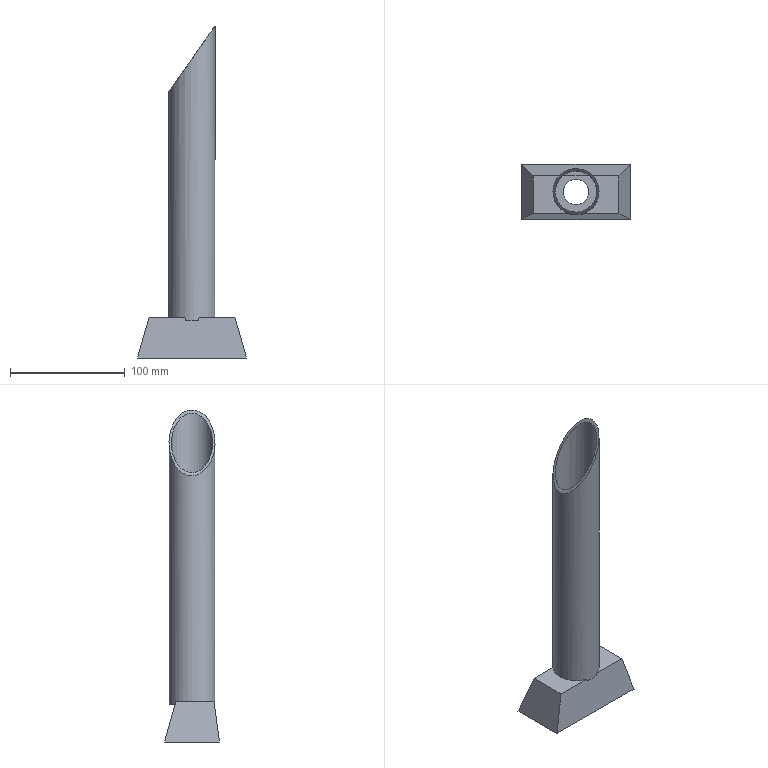Part | NX | features EXTRUDE 4, DATUM_CSYS 3, SKETCH 3, EXTRACT_DATUM_PLANE 2, SHELL 2, DRAFT 1, UNITE 1 | 1 solid | 19 faces | box 95 x 48 x 289.397 mm | volume 75187 mm3 | plane 12 | spline 4 | cylinder 3 | commonest cylinder face diameters 22.182 x1 36.182 x1 40.182 x1
STEP:
#1=CARTESIAN_POINT('',(5.362,-19.362,33.));
#2=VERTEX_POINT('',#1);
#3=CARTESIAN_POINT('',(6.29,-19.081,35.));
#4=VERTEX_POINT('',#3);
#5=CARTESIAN_POINT('',(0.,0.,170.769));
#6=DIRECTION('',(0.,0.9903,-0.1392));
#7=DIRECTION('',(0.,-0.1392,-0.9903));
#8=AXIS2_PLACEMENT_3D('',#5,#6,#7);
#9=ELLIPSE('',#8,144.36,20.091);
#10=EDGE_CURVE('',#2,#4,#9,.F.);
#11=ORIENTED_EDGE('',*,*,#10,.F.);
#12=CARTESIAN_POINT('',(-5.362,-19.362,33.));
#13=VERTEX_POINT('',#12);
#14=CARTESIAN_POINT('',(0.000000047,-19.362,33.));
#15=DIRECTION('',(1.,0.,0.));
#16=VECTOR('',#15,1000.);
#17=LINE('',#14,#16);
#18=EDGE_CURVE('',#13,#2,#17,.T.);
#19=ORIENTED_EDGE('',*,*,#18,.F.);
#20=CARTESIAN_POINT('',(-6.29,-19.081,35.));
#21=VERTEX_POINT('',#20);
#22=CARTESIAN_POINT('',(0.,0.,170.769));
#23=DIRECTION('',(0.,0.9903,-0.1392));
#24=DIRECTION('',(0.,-0.1392,-0.9903));
#25=AXIS2_PLACEMENT_3D('',#22,#23,#24);
#26=ELLIPSE('',#25,144.36,20.091);
#27=EDGE_CURVE('',#21,#13,#26,.F.);
#28=ORIENTED_EDGE('',*,*,#27,.F.);
#29=CARTESIAN_POINT('',(-37.464,-19.081,35.));
#30=VERTEX_POINT('',#29);
#31=CARTESIAN_POINT('',(0.000000047,-19.081,35.));
#32=DIRECTION('',(1.,0.,0.));
#33=VECTOR('',#32,1000.);
#34=LINE('',#31,#33);
#35=EDGE_CURVE('',#30,#21,#34,.T.);
#36=ORIENTED_EDGE('',*,*,#35,.F.);
#37=CARTESIAN_POINT('',(-47.5,-24.,0.));
#38=VERTEX_POINT('',#37);
#39=CARTESIAN_POINT('',(-37.464,-19.081,35.));
#40=CARTESIAN_POINT('',(-40.809,-20.721,23.333));
#41=CARTESIAN_POINT('',(-44.155,-22.36,11.667));
#42=CARTESIAN_POINT('',(-47.5,-24.,0.));
#43=B_SPLINE_CURVE_WITH_KNOTS('',3,(#39,#40,#41,#42),.UNSPECIFIED.,.F.,.F.,(4,4),(0.,0.03674),.UNSPECIFIED.);
#44=EDGE_CURVE('',#30,#38,#43,.T.);
#45=ORIENTED_EDGE('',*,*,#44,.T.);
#46=CARTESIAN_POINT('',(47.5,-24.,0.));
#47=VERTEX_POINT('',#46);
#48=CARTESIAN_POINT('',(0.000000047,-24.,0.));
#49=DIRECTION('',(1.,0.,0.));
#50=VECTOR('',#49,1000.);
#51=LINE('',#48,#50);
#52=EDGE_CURVE('',#38,#47,#51,.T.);
#53=ORIENTED_EDGE('',*,*,#52,.T.);
#54=CARTESIAN_POINT('',(37.463,-19.081,35.));
#55=VERTEX_POINT('',#54);
#56=CARTESIAN_POINT('',(37.463,-19.081,35.));
#57=CARTESIAN_POINT('',(40.809,-20.721,23.333));
#58=CARTESIAN_POINT('',(44.154,-22.36,11.667));
#59=CARTESIAN_POINT('',(47.5,-24.,0.));
#60=B_SPLINE_CURVE_WITH_KNOTS('',3,(#56,#57,#58,#59),.UNSPECIFIED.,.F.,.F.,(4,4),(0.,0.03674),.UNSPECIFIED.);
#61=EDGE_CURVE('',#55,#47,#60,.T.);
#62=ORIENTED_EDGE('',*,*,#61,.F.);
#63=CARTESIAN_POINT('',(0.000000047,-19.081,35.));
#64=DIRECTION('',(1.,0.,0.));
#65=VECTOR('',#64,1000.);
#66=LINE('',#63,#65);
#67=EDGE_CURVE('',#4,#55,#66,.T.);
#68=ORIENTED_EDGE('',*,*,#67,.F.);
#69=EDGE_LOOP('',(#11,#19,#28,#36,#45,#53,#62,#68));
#70=FACE_BOUND('',#69,.T.);
#71=CARTESIAN_POINT('',(0.000000047,-24.,0.));
#72=DIRECTION('',(0.,0.9903,-0.1392));
#73=DIRECTION('',(0.,0.1392,0.9903));
#74=AXIS2_PLACEMENT_3D('',#71,#72,#73);
#75=PLANE('',#74);
#76=ADVANCED_FACE('',(#70),#75,.F.);
#77=ORIENTED_EDGE('',*,*,#35,.T.);
#78=CARTESIAN_POINT('',(-14.445,13.964,35.));
#79=VERTEX_POINT('',#78);
#80=CARTESIAN_POINT('',(0.,0.,35.));
#81=DIRECTION('',(0.,0.,1.));
#82=DIRECTION('',(1.,0.,0.));
#83=AXIS2_PLACEMENT_3D('',#80,#81,#82);
#84=CIRCLE('',#83,20.091);
#85=EDGE_CURVE('',#21,#79,#84,.F.);
#86=ORIENTED_EDGE('',*,*,#85,.T.);
#87=CARTESIAN_POINT('',(-37.463,13.964,35.));
#88=VERTEX_POINT('',#87);
#89=CARTESIAN_POINT('',(0.000000047,13.964,35.));
#90=DIRECTION('',(-1.,0.,0.));
#91=VECTOR('',#90,1000.);
#92=LINE('',#89,#91);
#93=EDGE_CURVE('',#79,#88,#92,.T.);
#94=ORIENTED_EDGE('',*,*,#93,.T.);
#95=CARTESIAN_POINT('',(-37.463,13.964,35.));
#96=CARTESIAN_POINT('',(-37.463,2.949,35.));
#97=CARTESIAN_POINT('',(-37.463,-8.066,35.));
#98=CARTESIAN_POINT('',(-37.464,-19.081,35.));
#99=B_SPLINE_CURVE_WITH_KNOTS('',3,(#95,#96,#97,#98),.UNSPECIFIED.,.F.,.F.,(4,4),(0.,0.03304),.UNSPECIFIED.);
#100=EDGE_CURVE('',#88,#30,#99,.T.);
#101=ORIENTED_EDGE('',*,*,#100,.T.);
#102=EDGE_LOOP('',(#77,#86,#94,#101));
#103=FACE_BOUND('',#102,.T.);
#104=CARTESIAN_POINT('',(-47.5,-0.000000093,35.));
#105=DIRECTION('',(0.,0.,1.));
#106=DIRECTION('',(1.,0.,0.));
#107=AXIS2_PLACEMENT_3D('',#104,#105,#106);
#108=PLANE('',#107);
#109=ADVANCED_FACE('',(#103),#108,.T.);
#110=CARTESIAN_POINT('',(11.091,0.,35.));
#111=VERTEX_POINT('',#110);
#112=CARTESIAN_POINT('',(0.,0.,35.));
#113=DIRECTION('',(0.,0.,1.));
#114=DIRECTION('',(1.,0.,0.));
#115=AXIS2_PLACEMENT_3D('',#112,#113,#114);
#116=CIRCLE('',#115,11.091);
#117=EDGE_CURVE('',#111,#111,#116,.F.);
#118=ORIENTED_EDGE('',*,*,#117,.T.);
#119=EDGE_LOOP('',(#118));
#120=FACE_BOUND('',#119,.T.);
#121=CARTESIAN_POINT('',(11.502,13.964,35.));
#122=VERTEX_POINT('',#121);
#123=CARTESIAN_POINT('',(-11.502,13.964,35.));
#124=VERTEX_POINT('',#123);
#125=CARTESIAN_POINT('',(0.,0.,35.));
#126=DIRECTION('',(0.,0.,1.));
#127=DIRECTION('',(1.,0.,0.));
#128=AXIS2_PLACEMENT_3D('',#125,#126,#127);
#129=CIRCLE('',#128,18.091);
#130=EDGE_CURVE('',#122,#124,#129,.F.);
#131=ORIENTED_EDGE('',*,*,#130,.F.);
#132=CARTESIAN_POINT('',(0.000000047,13.964,35.));
#133=DIRECTION('',(-1.,0.,0.));
#134=VECTOR('',#133,1000.);
#135=LINE('',#132,#134);
#136=EDGE_CURVE('',#122,#124,#135,.T.);
#137=ORIENTED_EDGE('',*,*,#136,.T.);
#138=EDGE_LOOP('',(#131,#137));
#139=FACE_BOUND('',#138,.T.);
#140=CARTESIAN_POINT('',(-47.5,-0.000000093,35.));
#141=DIRECTION('',(0.,0.,1.));
#142=DIRECTION('',(1.,0.,0.));
#143=AXIS2_PLACEMENT_3D('',#140,#141,#142);
#144=PLANE('',#143);
#145=ADVANCED_FACE('',(#120,#139),#144,.T.);
#146=CARTESIAN_POINT('',(-13.868,14.537,33.));
#147=VERTEX_POINT('',#146);
#148=CARTESIAN_POINT('',(0.,0.,83.698));
#149=DIRECTION('',(0.,-0.9613,-0.2756));
#150=DIRECTION('',(0.,0.2756,-0.9613));
#151=AXIS2_PLACEMENT_3D('',#148,#149,#150);
#152=ELLIPSE('',#151,72.889,20.091);
#153=EDGE_CURVE('',#147,#79,#152,.F.);
#154=ORIENTED_EDGE('',*,*,#153,.F.);
#155=CARTESIAN_POINT('',(-10.768,14.537,33.));
#156=VERTEX_POINT('',#155);
#157=CARTESIAN_POINT('',(0.000000047,14.537,33.));
#158=DIRECTION('',(-1.,0.,0.));
#159=VECTOR('',#158,1000.);
#160=LINE('',#157,#159);
#161=EDGE_CURVE('',#156,#147,#160,.T.);
#162=ORIENTED_EDGE('',*,*,#161,.F.);
#163=CARTESIAN_POINT('',(0.,0.,83.698));
#164=DIRECTION('',(0.,-0.9613,-0.2756));
#165=DIRECTION('',(0.,0.2756,-0.9613));
#166=AXIS2_PLACEMENT_3D('',#163,#164,#165);
#167=ELLIPSE('',#166,65.633,18.091);
#168=EDGE_CURVE('',#124,#156,#167,.T.);
#169=ORIENTED_EDGE('',*,*,#168,.F.);
#170=ORIENTED_EDGE('',*,*,#136,.F.);
#171=CARTESIAN_POINT('',(10.768,14.537,33.));
#172=VERTEX_POINT('',#171);
#173=CARTESIAN_POINT('',(0.,0.,83.698));
#174=DIRECTION('',(0.,-0.9613,-0.2756));
#175=DIRECTION('',(0.,0.2756,-0.9613));
#176=AXIS2_PLACEMENT_3D('',#173,#174,#175);
#177=ELLIPSE('',#176,65.633,18.091);
#178=EDGE_CURVE('',#172,#122,#177,.T.);
#179=ORIENTED_EDGE('',*,*,#178,.F.);
#180=CARTESIAN_POINT('',(13.868,14.537,33.));
#181=VERTEX_POINT('',#180);
#182=CARTESIAN_POINT('',(0.000000047,14.537,33.));
#183=DIRECTION('',(-1.,0.,0.));
#184=VECTOR('',#183,1000.);
#185=LINE('',#182,#184);
#186=EDGE_CURVE('',#181,#172,#185,.T.);
#187=ORIENTED_EDGE('',*,*,#186,.F.);
#188=CARTESIAN_POINT('',(14.445,13.964,35.));
#189=VERTEX_POINT('',#188);
#190=CARTESIAN_POINT('',(0.,0.,83.698));
#191=DIRECTION('',(0.,-0.9613,-0.2756));
#192=DIRECTION('',(0.,0.2756,-0.9613));
#193=AXIS2_PLACEMENT_3D('',#190,#191,#192);
#194=ELLIPSE('',#193,72.889,20.091);
#195=EDGE_CURVE('',#189,#181,#194,.F.);
#196=ORIENTED_EDGE('',*,*,#195,.F.);
#197=CARTESIAN_POINT('',(37.463,13.964,35.));
#198=VERTEX_POINT('',#197);
#199=CARTESIAN_POINT('',(0.000000047,13.964,35.));
#200=DIRECTION('',(-1.,0.,0.));
#201=VECTOR('',#200,1000.);
#202=LINE('',#199,#201);
#203=EDGE_CURVE('',#198,#189,#202,.T.);
#204=ORIENTED_EDGE('',*,*,#203,.F.);
#205=CARTESIAN_POINT('',(47.5,24.,0.));
#206=VERTEX_POINT('',#205);
#207=CARTESIAN_POINT('',(37.463,13.964,35.));
#208=CARTESIAN_POINT('',(40.809,17.309,23.333));
#209=CARTESIAN_POINT('',(44.154,20.655,11.667));
#210=CARTESIAN_POINT('',(47.5,24.,0.));
#211=B_SPLINE_CURVE_WITH_KNOTS('',3,(#207,#208,#209,#210),.UNSPECIFIED.,.F.,.F.,(4,4),(0.,0.03777),.UNSPECIFIED.);
#212=EDGE_CURVE('',#198,#206,#211,.T.);
#213=ORIENTED_EDGE('',*,*,#212,.T.);
#214=CARTESIAN_POINT('',(-47.5,24.,0.));
#215=VERTEX_POINT('',#214);
#216=CARTESIAN_POINT('',(0.000000047,24.,0.));
#217=DIRECTION('',(-1.,0.,0.));
#218=VECTOR('',#217,1000.);
#219=LINE('',#216,#218);
#220=EDGE_CURVE('',#206,#215,#219,.T.);
#221=ORIENTED_EDGE('',*,*,#220,.T.);
#222=CARTESIAN_POINT('',(-37.463,13.964,35.));
#223=CARTESIAN_POINT('',(-40.809,17.309,23.333));
#224=CARTESIAN_POINT('',(-44.154,20.655,11.667));
#225=CARTESIAN_POINT('',(-47.5,24.,0.));
#226=B_SPLINE_CURVE_WITH_KNOTS('',3,(#222,#223,#224,#225),.UNSPECIFIED.,.F.,.F.,(4,4),(0.,0.03777),.UNSPECIFIED.);
#227=EDGE_CURVE('',#88,#215,#226,.T.);
#228=ORIENTED_EDGE('',*,*,#227,.F.);
#229=ORIENTED_EDGE('',*,*,#93,.F.);
#230=EDGE_LOOP('',(#154,#162,#169,#170,#179,#187,#196,#204,#213,#221,#228,#229));
#231=FACE_BOUND('',#230,.T.);
#232=CARTESIAN_POINT('',(0.000000047,24.,0.));
#233=DIRECTION('',(0.,-0.9613,-0.2756));
#234=DIRECTION('',(0.,0.2756,-0.9613));
#235=AXIS2_PLACEMENT_3D('',#232,#233,#234);
#236=PLANE('',#235);
#237=ADVANCED_FACE('',(#231),#236,.F.);
#238=CARTESIAN_POINT('',(-47.5,24.,0.));
#239=CARTESIAN_POINT('',(-47.498,8.,0.));
#240=CARTESIAN_POINT('',(-47.499,-8.,0.));
#241=CARTESIAN_POINT('',(-47.5,-24.,0.));
#242=B_SPLINE_CURVE_WITH_KNOTS('',3,(#238,#239,#240,#241),.UNSPECIFIED.,.F.,.F.,(4,4),(0.,0.048),.UNSPECIFIED.);
#243=EDGE_CURVE('',#215,#38,#242,.T.);
#244=ORIENTED_EDGE('',*,*,#243,.T.);
#245=ORIENTED_EDGE('',*,*,#44,.F.);
#246=ORIENTED_EDGE('',*,*,#100,.F.);
#247=ORIENTED_EDGE('',*,*,#227,.T.);
#248=EDGE_LOOP('',(#244,#245,#246,#247));
#249=FACE_BOUND('',#248,.T.);
#250=CARTESIAN_POINT('',(-37.464,24.001,35.));
#251=CARTESIAN_POINT('',(-37.462,7.909,35.));
#252=CARTESIAN_POINT('',(-37.462,-8.197,35.));
#253=CARTESIAN_POINT('',(-37.464,-24.289,35.));
#254=CARTESIAN_POINT('',(-47.5,24.,0.));
#255=CARTESIAN_POINT('',(-47.498,7.911,0.));
#256=CARTESIAN_POINT('',(-47.499,-8.199,0.));
#257=CARTESIAN_POINT('',(-47.5,-24.288,0.));
#258=B_SPLINE_SURFACE_WITH_KNOTS('',1,3,((#250,#251,#252,#253),(#254,#255,#256,#257)),.RULED_SURF.,.F.,.F.,.F.,(2,2),(4,4),(0.1667,1.),(0.,1.006),.PIECEWISE_BEZIER_KNOTS.);
#259=ADVANCED_FACE('',(#249),#258,.T.);
#260=CARTESIAN_POINT('',(47.5,-24.,0.));
#261=CARTESIAN_POINT('',(47.498,-8.,0.));
#262=CARTESIAN_POINT('',(47.499,8.,0.));
#263=CARTESIAN_POINT('',(47.5,24.,0.));
#264=B_SPLINE_CURVE_WITH_KNOTS('',3,(#260,#261,#262,#263),.UNSPECIFIED.,.F.,.F.,(4,4),(0.,0.048),.UNSPECIFIED.);
#265=EDGE_CURVE('',#47,#206,#264,.T.);
#266=ORIENTED_EDGE('',*,*,#265,.T.);
#267=ORIENTED_EDGE('',*,*,#212,.F.);
#268=CARTESIAN_POINT('',(37.463,-19.081,35.));
#269=CARTESIAN_POINT('',(37.463,-8.066,35.));
#270=CARTESIAN_POINT('',(37.463,2.949,35.));
#271=CARTESIAN_POINT('',(37.463,13.964,35.));
#272=B_SPLINE_CURVE_WITH_KNOTS('',3,(#268,#269,#270,#271),.UNSPECIFIED.,.F.,.F.,(4,4),(0.,0.03304),.UNSPECIFIED.);
#273=EDGE_CURVE('',#55,#198,#272,.T.);
#274=ORIENTED_EDGE('',*,*,#273,.F.);
#275=ORIENTED_EDGE('',*,*,#61,.T.);
#276=EDGE_LOOP('',(#266,#267,#274,#275));
#277=FACE_BOUND('',#276,.T.);
#278=CARTESIAN_POINT('',(37.464,-24.001,35.));
#279=CARTESIAN_POINT('',(37.462,-7.909,35.));
#280=CARTESIAN_POINT('',(37.462,8.197,35.));
#281=CARTESIAN_POINT('',(37.464,24.289,35.));
#282=CARTESIAN_POINT('',(47.5,-24.,0.));
#283=CARTESIAN_POINT('',(47.498,-7.911,0.));
#284=CARTESIAN_POINT('',(47.499,8.199,0.));
#285=CARTESIAN_POINT('',(47.5,24.288,0.));
#286=B_SPLINE_SURFACE_WITH_KNOTS('',1,3,((#278,#279,#280,#281),(#282,#283,#284,#285)),.RULED_SURF.,.F.,.F.,.F.,(2,2),(4,4),(0.1667,1.),(0.,1.006),.PIECEWISE_BEZIER_KNOTS.);
#287=ADVANCED_FACE('',(#277),#286,.T.);
#288=ORIENTED_EDGE('',*,*,#203,.T.);
#289=CARTESIAN_POINT('',(0.,0.,35.));
#290=DIRECTION('',(0.,0.,1.));
#291=DIRECTION('',(1.,0.,0.));
#292=AXIS2_PLACEMENT_3D('',#289,#290,#291);
#293=CIRCLE('',#292,20.091);
#294=EDGE_CURVE('',#189,#4,#293,.F.);
#295=ORIENTED_EDGE('',*,*,#294,.T.);
#296=ORIENTED_EDGE('',*,*,#67,.T.);
#297=ORIENTED_EDGE('',*,*,#273,.T.);
#298=EDGE_LOOP('',(#288,#295,#296,#297));
#299=FACE_BOUND('',#298,.T.);
#300=CARTESIAN_POINT('',(-47.5,-0.000000093,35.));
#301=DIRECTION('',(0.,0.,1.));
#302=DIRECTION('',(1.,0.,0.));
#303=AXIS2_PLACEMENT_3D('',#300,#301,#302);
#304=PLANE('',#303);
#305=ADVANCED_FACE('',(#299),#304,.T.);
#306=CARTESIAN_POINT('',(45.419,-21.98,0.));
#307=VERTEX_POINT('',#306);
#308=CARTESIAN_POINT('',(45.419,21.919,0.));
#309=VERTEX_POINT('',#308);
#310=CARTESIAN_POINT('',(45.419,-21.98,0.));
#311=CARTESIAN_POINT('',(45.418,-7.347,0.));
#312=CARTESIAN_POINT('',(45.418,7.286,0.));
#313=CARTESIAN_POINT('',(45.419,21.919,0.));
#314=B_SPLINE_CURVE_WITH_KNOTS('',3,(#310,#311,#312,#313),.UNSPECIFIED.,.F.,.F.,(4,4),(0.,0.0439),.UNSPECIFIED.);
#315=EDGE_CURVE('',#307,#309,#314,.T.);
#316=ORIENTED_EDGE('',*,*,#315,.T.);
#317=CARTESIAN_POINT('',(-45.419,21.919,0.));
#318=VERTEX_POINT('',#317);
#319=CARTESIAN_POINT('',(0.000000047,21.919,0.));
#320=DIRECTION('',(-1.,0.,0.));
#321=VECTOR('',#320,1000.);
#322=LINE('',#319,#321);
#323=EDGE_CURVE('',#309,#318,#322,.T.);
#324=ORIENTED_EDGE('',*,*,#323,.T.);
#325=CARTESIAN_POINT('',(-45.419,-21.98,0.));
#326=VERTEX_POINT('',#325);
#327=CARTESIAN_POINT('',(-45.419,21.919,0.));
#328=CARTESIAN_POINT('',(-45.418,7.286,0.));
#329=CARTESIAN_POINT('',(-45.418,-7.347,0.));
#330=CARTESIAN_POINT('',(-45.419,-21.98,0.));
#331=B_SPLINE_CURVE_WITH_KNOTS('',3,(#327,#328,#329,#330),.UNSPECIFIED.,.F.,.F.,(4,4),(0.,0.0439),.UNSPECIFIED.);
#332=EDGE_CURVE('',#318,#326,#331,.T.);
#333=ORIENTED_EDGE('',*,*,#332,.T.);
#334=CARTESIAN_POINT('',(0.000000047,-21.98,0.));
#335=DIRECTION('',(1.,0.,0.));
#336=VECTOR('',#335,1000.);
#337=LINE('',#334,#336);
#338=EDGE_CURVE('',#326,#307,#337,.T.);
#339=ORIENTED_EDGE('',*,*,#338,.T.);
#340=EDGE_LOOP('',(#316,#324,#333,#339));
#341=FACE_BOUND('',#340,.T.);
#342=ORIENTED_EDGE('',*,*,#220,.F.);
#343=ORIENTED_EDGE('',*,*,#265,.F.);
#344=ORIENTED_EDGE('',*,*,#52,.F.);
#345=ORIENTED_EDGE('',*,*,#243,.F.);
#346=EDGE_LOOP('',(#342,#343,#344,#345));
#347=FACE_BOUND('',#346,.T.);
#348=CARTESIAN_POINT('',(-47.5,-0.000000093,0.));
#349=DIRECTION('',(0.,0.,1.));
#350=DIRECTION('',(1.,0.,0.));
#351=AXIS2_PLACEMENT_3D('',#348,#349,#350);
#352=PLANE('',#351);
#353=ADVANCED_FACE('',(#341,#347),#352,.F.);
#354=ORIENTED_EDGE('',*,*,#323,.F.);
#355=CARTESIAN_POINT('',(35.956,12.457,33.));
#356=VERTEX_POINT('',#355);
#357=CARTESIAN_POINT('',(35.956,12.457,33.));
#358=CARTESIAN_POINT('',(39.11,15.611,22.));
#359=CARTESIAN_POINT('',(42.265,18.765,11.));
#360=CARTESIAN_POINT('',(45.419,21.919,0.));
#361=B_SPLINE_CURVE_WITH_KNOTS('',3,(#357,#358,#359,#360),.UNSPECIFIED.,.F.,.F.,(4,4),(0.,0.03561),.UNSPECIFIED.);
#362=EDGE_CURVE('',#356,#309,#361,.T.);
#363=ORIENTED_EDGE('',*,*,#362,.F.);
#364=CARTESIAN_POINT('',(-35.956,12.457,33.));
#365=VERTEX_POINT('',#364);
#366=CARTESIAN_POINT('',(0.000000047,12.457,33.));
#367=DIRECTION('',(-1.,0.,0.));
#368=VECTOR('',#367,1000.);
#369=LINE('',#366,#368);
#370=EDGE_CURVE('',#356,#365,#369,.T.);
#371=ORIENTED_EDGE('',*,*,#370,.T.);
#372=CARTESIAN_POINT('',(-35.956,12.457,33.));
#373=CARTESIAN_POINT('',(-39.11,15.611,22.));
#374=CARTESIAN_POINT('',(-42.265,18.765,11.));
#375=CARTESIAN_POINT('',(-45.419,21.919,0.));
#376=B_SPLINE_CURVE_WITH_KNOTS('',3,(#372,#373,#374,#375),.UNSPECIFIED.,.F.,.F.,(4,4),(0.,0.03561),.UNSPECIFIED.);
#377=EDGE_CURVE('',#365,#318,#376,.T.);
#378=ORIENTED_EDGE('',*,*,#377,.T.);
#379=EDGE_LOOP('',(#354,#363,#371,#378));
#380=FACE_BOUND('',#379,.T.);
#381=CARTESIAN_POINT('',(0.000000047,22.077,-0.5513));
#382=DIRECTION('',(0.,-0.9613,-0.2756));
#383=DIRECTION('',(0.,0.2756,-0.9613));
#384=AXIS2_PLACEMENT_3D('',#381,#382,#383);
#385=PLANE('',#384);
#386=ADVANCED_FACE('',(#380),#385,.T.);
#387=ORIENTED_EDGE('',*,*,#332,.F.);
#388=ORIENTED_EDGE('',*,*,#377,.F.);
#389=CARTESIAN_POINT('',(-35.956,-17.342,33.));
#390=VERTEX_POINT('',#389);
#391=CARTESIAN_POINT('',(-35.956,12.457,33.));
#392=CARTESIAN_POINT('',(-35.955,2.524,33.));
#393=CARTESIAN_POINT('',(-35.956,-7.409,33.));
#394=CARTESIAN_POINT('',(-35.956,-17.342,33.));
#395=B_SPLINE_CURVE_WITH_KNOTS('',3,(#391,#392,#393,#394),.UNSPECIFIED.,.F.,.F.,(4,4),(0.,0.0298),.UNSPECIFIED.);
#396=EDGE_CURVE('',#365,#390,#395,.T.);
#397=ORIENTED_EDGE('',*,*,#396,.T.);
#398=CARTESIAN_POINT('',(-35.956,-17.342,33.));
#399=CARTESIAN_POINT('',(-39.111,-18.888,22.));
#400=CARTESIAN_POINT('',(-42.265,-20.434,11.));
#401=CARTESIAN_POINT('',(-45.419,-21.98,0.));
#402=B_SPLINE_CURVE_WITH_KNOTS('',3,(#398,#399,#400,#401),.UNSPECIFIED.,.F.,.F.,(4,4),(0.,0.03464),.UNSPECIFIED.);
#403=EDGE_CURVE('',#390,#326,#402,.T.);
#404=ORIENTED_EDGE('',*,*,#403,.T.);
#405=EDGE_LOOP('',(#387,#388,#397,#404));
#406=FACE_BOUND('',#405,.T.);
#407=CARTESIAN_POINT('',(-35.957,22.183,33.));
#408=CARTESIAN_POINT('',(-35.955,7.378,33.));
#409=CARTESIAN_POINT('',(-35.955,-7.439,33.));
#410=CARTESIAN_POINT('',(-35.957,-22.244,33.));
#411=CARTESIAN_POINT('',(-39.111,22.183,22.));
#412=CARTESIAN_POINT('',(-39.109,7.378,22.));
#413=CARTESIAN_POINT('',(-39.11,-7.439,22.));
#414=CARTESIAN_POINT('',(-39.111,-22.244,22.));
#415=CARTESIAN_POINT('',(-42.265,22.183,11.));
#416=CARTESIAN_POINT('',(-42.264,7.379,11.));
#417=CARTESIAN_POINT('',(-42.264,-7.44,11.));
#418=CARTESIAN_POINT('',(-42.265,-22.244,11.));
#419=CARTESIAN_POINT('',(-45.419,22.183,0.));
#420=CARTESIAN_POINT('',(-45.418,7.379,-0.000000013));
#421=CARTESIAN_POINT('',(-45.418,-7.44,-0.000000012));
#422=CARTESIAN_POINT('',(-45.419,-22.244,0.));
#423=B_SPLINE_SURFACE_WITH_KNOTS('',3,3,((#407,#408,#409,#410),(#411,#412,#413,#414),(#415,#416,#417,#418),(#419,#420,#421,#422)),.UNSPECIFIED.,.F.,.F.,.F.,(4,4),(4,4),(0.2012,0.9869),(0.03788,0.9634),.UNSPECIFIED.);
#424=ADVANCED_FACE('',(#406),#423,.F.);
#425=ORIENTED_EDGE('',*,*,#338,.F.);
#426=ORIENTED_EDGE('',*,*,#403,.F.);
#427=CARTESIAN_POINT('',(35.956,-17.342,33.));
#428=VERTEX_POINT('',#427);
#429=CARTESIAN_POINT('',(0.000000047,-17.342,33.));
#430=DIRECTION('',(1.,0.,0.));
#431=VECTOR('',#430,1000.);
#432=LINE('',#429,#431);
#433=EDGE_CURVE('',#390,#428,#432,.T.);
#434=ORIENTED_EDGE('',*,*,#433,.T.);
#435=CARTESIAN_POINT('',(35.956,-17.342,33.));
#436=CARTESIAN_POINT('',(39.111,-18.888,22.));
#437=CARTESIAN_POINT('',(42.265,-20.434,11.));
#438=CARTESIAN_POINT('',(45.419,-21.98,0.));
#439=B_SPLINE_CURVE_WITH_KNOTS('',3,(#435,#436,#437,#438),.UNSPECIFIED.,.F.,.F.,(4,4),(0.,0.03464),.UNSPECIFIED.);
#440=EDGE_CURVE('',#428,#307,#439,.T.);
#441=ORIENTED_EDGE('',*,*,#440,.T.);
#442=EDGE_LOOP('',(#425,#426,#434,#441));
#443=FACE_BOUND('',#442,.T.);
#444=CARTESIAN_POINT('',(0.000000047,-22.019,-0.2783));
#445=DIRECTION('',(0.,0.9903,-0.1392));
#446=DIRECTION('',(0.,0.1392,0.9903));
#447=AXIS2_PLACEMENT_3D('',#444,#445,#446);
#448=PLANE('',#447);
#449=ADVANCED_FACE('',(#443),#448,.T.);
#450=ORIENTED_EDGE('',*,*,#315,.F.);
#451=ORIENTED_EDGE('',*,*,#440,.F.);
#452=CARTESIAN_POINT('',(35.956,-17.342,33.));
#453=CARTESIAN_POINT('',(35.956,-7.409,33.));
#454=CARTESIAN_POINT('',(35.955,2.524,33.));
#455=CARTESIAN_POINT('',(35.956,12.457,33.));
#456=B_SPLINE_CURVE_WITH_KNOTS('',3,(#452,#453,#454,#455),.UNSPECIFIED.,.F.,.F.,(4,4),(0.,0.0298),.UNSPECIFIED.);
#457=EDGE_CURVE('',#428,#356,#456,.T.);
#458=ORIENTED_EDGE('',*,*,#457,.T.);
#459=ORIENTED_EDGE('',*,*,#362,.T.);
#460=EDGE_LOOP('',(#450,#451,#458,#459));
#461=FACE_BOUND('',#460,.T.);
#462=CARTESIAN_POINT('',(35.957,-22.244,33.));
#463=CARTESIAN_POINT('',(35.955,-7.439,33.));
#464=CARTESIAN_POINT('',(35.955,7.378,33.));
#465=CARTESIAN_POINT('',(35.957,22.183,33.));
#466=CARTESIAN_POINT('',(39.111,-22.244,22.));
#467=CARTESIAN_POINT('',(39.109,-7.439,22.));
#468=CARTESIAN_POINT('',(39.11,7.378,22.));
#469=CARTESIAN_POINT('',(39.111,22.183,22.));
#470=CARTESIAN_POINT('',(42.265,-22.244,11.));
#471=CARTESIAN_POINT('',(42.264,-7.44,11.));
#472=CARTESIAN_POINT('',(42.264,7.379,11.));
#473=CARTESIAN_POINT('',(42.265,22.183,11.));
#474=CARTESIAN_POINT('',(45.419,-22.244,0.));
#475=CARTESIAN_POINT('',(45.418,-7.44,-0.000000013));
#476=CARTESIAN_POINT('',(45.418,7.379,-0.000000012));
#477=CARTESIAN_POINT('',(45.419,22.183,0.));
#478=B_SPLINE_SURFACE_WITH_KNOTS('',3,3,((#462,#463,#464,#465),(#466,#467,#468,#469),(#470,#471,#472,#473),(#474,#475,#476,#477)),.UNSPECIFIED.,.F.,.F.,.F.,(4,4),(4,4),(0.2012,0.9869),(0.03661,0.9621),.UNSPECIFIED.);
#479=ADVANCED_FACE('',(#461),#478,.F.);
#480=ORIENTED_EDGE('',*,*,#457,.F.);
#481=ORIENTED_EDGE('',*,*,#433,.F.);
#482=ORIENTED_EDGE('',*,*,#396,.F.);
#483=ORIENTED_EDGE('',*,*,#370,.F.);
#484=EDGE_LOOP('',(#480,#481,#482,#483));
#485=FACE_BOUND('',#484,.T.);
#486=CARTESIAN_POINT('',(11.091,0.,33.));
#487=VERTEX_POINT('',#486);
#488=CARTESIAN_POINT('',(0.,0.,33.));
#489=DIRECTION('',(0.,0.,1.));
#490=DIRECTION('',(1.,0.,0.));
#491=AXIS2_PLACEMENT_3D('',#488,#489,#490);
#492=CIRCLE('',#491,11.091);
#493=EDGE_CURVE('',#487,#487,#492,.F.);
#494=ORIENTED_EDGE('',*,*,#493,.F.);
#495=EDGE_LOOP('',(#494));
#496=FACE_BOUND('',#495,.T.);
#497=CARTESIAN_POINT('',(-47.5,-0.000000093,33.));
#498=DIRECTION('',(0.,0.,1.));
#499=DIRECTION('',(1.,0.,0.));
#500=AXIS2_PLACEMENT_3D('',#497,#498,#499);
#501=PLANE('',#500);
#502=ADVANCED_FACE('',(#485,#496),#501,.F.);
#503=ORIENTED_EDGE('',*,*,#117,.F.);
#504=EDGE_LOOP('',(#503));
#505=FACE_BOUND('',#504,.T.);
#506=ORIENTED_EDGE('',*,*,#493,.T.);
#507=EDGE_LOOP('',(#506));
#508=FACE_BOUND('',#507,.T.);
#509=CARTESIAN_POINT('',(0.,0.,292.));
#510=DIRECTION('',(0.,0.,-1.));
#511=DIRECTION('',(-1.,0.,0.));
#512=AXIS2_PLACEMENT_3D('',#509,#510,#511);
#513=CYLINDRICAL_SURFACE('',#512,11.091);
#514=ADVANCED_FACE('',(#505,#508),#513,.F.);
#515=CARTESIAN_POINT('',(0.,0.,33.));
#516=DIRECTION('',(0.,0.,1.));
#517=DIRECTION('',(-1.,0.,0.));
#518=AXIS2_PLACEMENT_3D('',#515,#516,#517);
#519=CIRCLE('',#518,20.091);
#520=EDGE_CURVE('',#181,#147,#519,.T.);
#521=ORIENTED_EDGE('',*,*,#520,.F.);
#522=ORIENTED_EDGE('',*,*,#186,.T.);
#523=CARTESIAN_POINT('',(0.,0.,33.));
#524=DIRECTION('',(0.,0.,1.));
#525=DIRECTION('',(1.,0.,0.));
#526=AXIS2_PLACEMENT_3D('',#523,#524,#525);
#527=CIRCLE('',#526,18.091);
#528=EDGE_CURVE('',#172,#156,#527,.T.);
#529=ORIENTED_EDGE('',*,*,#528,.T.);
#530=ORIENTED_EDGE('',*,*,#161,.T.);
#531=EDGE_LOOP('',(#521,#522,#529,#530));
#532=FACE_BOUND('',#531,.T.);
#533=CARTESIAN_POINT('',(0.,0.,33.));
#534=DIRECTION('',(0.,0.,1.));
#535=DIRECTION('',(1.,0.,0.));
#536=AXIS2_PLACEMENT_3D('',#533,#534,#535);
#537=PLANE('',#536);
#538=ADVANCED_FACE('',(#532),#537,.F.);
#539=CARTESIAN_POINT('',(0.,0.,33.));
#540=DIRECTION('',(0.,0.,1.));
#541=DIRECTION('',(-1.,0.,0.));
#542=AXIS2_PLACEMENT_3D('',#539,#540,#541);
#543=CIRCLE('',#542,20.091);
#544=EDGE_CURVE('',#13,#2,#543,.T.);
#545=ORIENTED_EDGE('',*,*,#544,.F.);
#546=ORIENTED_EDGE('',*,*,#18,.T.);
#547=EDGE_LOOP('',(#545,#546));
#548=FACE_BOUND('',#547,.T.);
#549=CARTESIAN_POINT('',(0.,0.,33.));
#550=DIRECTION('',(0.,0.,1.));
#551=DIRECTION('',(1.,0.,0.));
#552=AXIS2_PLACEMENT_3D('',#549,#550,#551);
#553=PLANE('',#552);
#554=ADVANCED_FACE('',(#548),#553,.F.);
#555=CARTESIAN_POINT('',(-20.091,0.,232.011));
#556=VERTEX_POINT('',#555);
#557=CARTESIAN_POINT('',(0.,0.,260.704));
#558=DIRECTION('',(0.8192,0.,-0.5736));
#559=DIRECTION('',(-0.5736,0.,-0.8192));
#560=AXIS2_PLACEMENT_3D('',#557,#558,#559);
#561=ELLIPSE('',#560,35.028,20.091);
#562=EDGE_CURVE('',#556,#556,#561,.T.);
#563=ORIENTED_EDGE('',*,*,#562,.T.);
#564=EDGE_LOOP('',(#563));
#565=FACE_BOUND('',#564,.T.);
#566=ORIENTED_EDGE('',*,*,#520,.T.);
#567=ORIENTED_EDGE('',*,*,#153,.T.);
#568=ORIENTED_EDGE('',*,*,#85,.F.);
#569=ORIENTED_EDGE('',*,*,#27,.T.);
#570=ORIENTED_EDGE('',*,*,#544,.T.);
#571=ORIENTED_EDGE('',*,*,#10,.T.);
#572=ORIENTED_EDGE('',*,*,#294,.F.);
#573=ORIENTED_EDGE('',*,*,#195,.T.);
#574=EDGE_LOOP('',(#566,#567,#568,#569,#570,#571,#572,#573));
#575=FACE_BOUND('',#574,.T.);
#576=CARTESIAN_POINT('',(0.,0.,292.));
#577=DIRECTION('',(0.,0.,-1.));
#578=DIRECTION('',(-1.,0.,0.));
#579=AXIS2_PLACEMENT_3D('',#576,#577,#578);
#580=CYLINDRICAL_SURFACE('',#579,20.091);
#581=ADVANCED_FACE('',(#565,#575),#580,.T.);
#582=CARTESIAN_POINT('',(-18.091,0.,234.867));
#583=VERTEX_POINT('',#582);
#584=CARTESIAN_POINT('',(0.,0.,260.704));
#585=DIRECTION('',(0.8192,0.,-0.5736));
#586=DIRECTION('',(-0.5736,0.,-0.8192));
#587=AXIS2_PLACEMENT_3D('',#584,#585,#586);
#588=ELLIPSE('',#587,31.541,18.091);
#589=EDGE_CURVE('',#583,#583,#588,.T.);
#590=ORIENTED_EDGE('',*,*,#589,.F.);
#591=EDGE_LOOP('',(#590));
#592=FACE_BOUND('',#591,.T.);
#593=ORIENTED_EDGE('',*,*,#168,.T.);
#594=ORIENTED_EDGE('',*,*,#528,.F.);
#595=ORIENTED_EDGE('',*,*,#178,.T.);
#596=ORIENTED_EDGE('',*,*,#130,.T.);
#597=EDGE_LOOP('',(#593,#594,#595,#596));
#598=FACE_BOUND('',#597,.T.);
#599=CARTESIAN_POINT('',(0.,0.,292.));
#600=DIRECTION('',(0.,0.,-1.));
#601=DIRECTION('',(-1.,0.,0.));
#602=AXIS2_PLACEMENT_3D('',#599,#600,#601);
#603=CYLINDRICAL_SURFACE('',#602,18.091);
#604=ADVANCED_FACE('',(#592,#598),#603,.F.);
#605=ORIENTED_EDGE('',*,*,#589,.T.);
#606=EDGE_LOOP('',(#605));
#607=FACE_BOUND('',#606,.T.);
#608=ORIENTED_EDGE('',*,*,#562,.F.);
#609=EDGE_LOOP('',(#608));
#610=FACE_BOUND('',#609,.T.);
#611=CARTESIAN_POINT('',(-25.,134.203,225.));
#612=DIRECTION('',(0.8192,0.,-0.5736));
#613=DIRECTION('',(-0.5736,0.,-0.8192));
#614=AXIS2_PLACEMENT_3D('',#611,#612,#613);
#615=PLANE('',#614);
#616=ADVANCED_FACE('',(#607,#610),#615,.F.);
#617=CLOSED_SHELL('',(#76,#109,#145,#237,#259,#287,#305,#353,#386,#424,#449,#479,#502,#514,#538,#554,#581,#604,#616));
#618=MANIFOLD_SOLID_BREP('',#617);
#619=(LENGTH_UNIT()NAMED_UNIT(*)SI_UNIT(.MILLI.,.METRE.));
#620=UNCERTAINTY_MEASURE_WITH_UNIT(LENGTH_MEASURE(0.0508),#619,'','');
#621=(NAMED_UNIT(*)PLANE_ANGLE_UNIT()SI_UNIT($,.RADIAN.));
#622=(NAMED_UNIT(*)SI_UNIT($,.STERADIAN.)SOLID_ANGLE_UNIT());
#623=(GEOMETRIC_REPRESENTATION_CONTEXT(3)GLOBAL_UNCERTAINTY_ASSIGNED_CONTEXT((#620))GLOBAL_UNIT_ASSIGNED_CONTEXT((#619,#621,#622))REPRESENTATION_CONTEXT('',''));
#624=ADVANCED_BREP_SHAPE_REPRESENTATION('',(#618),#623);